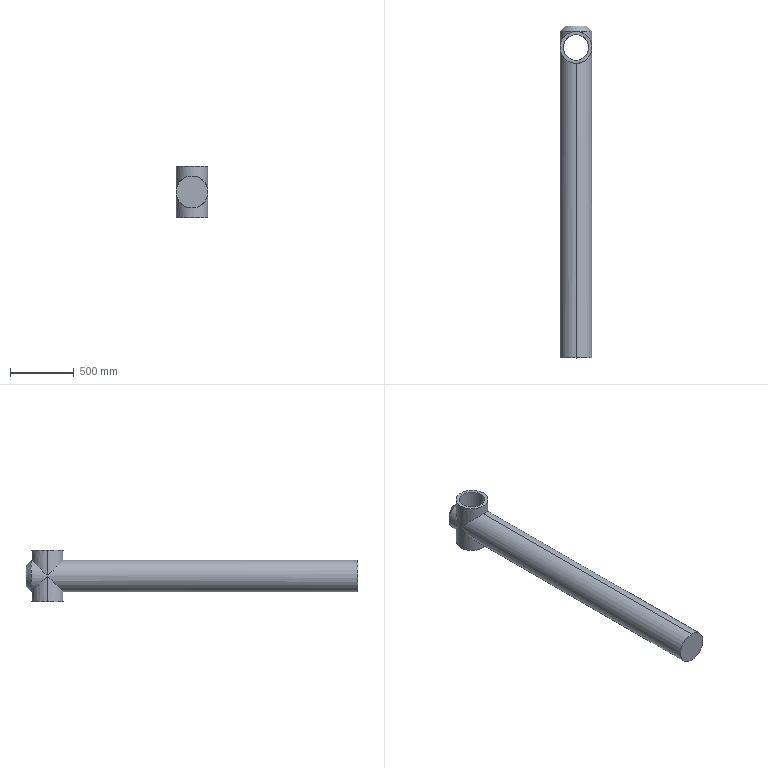Part | SolidWorks | features ICE 3, Chamfer 1, Extrusion 1 | 1 solid | 16 faces | box 250 x 2600 x 400 mm | volume 123717822 mm3 | cylinder 10 | plane 4 | cone 2 | commonest cylinder face diameters 250 x8 200 x2
STEP:
#1=CARTESIAN_POINT('',(0.,4000.,85.));
#2=VERTEX_POINT('',#1);
#3=CARTESIAN_POINT('',(0.,4000.,-85.));
#4=VERTEX_POINT('',#3);
#5=CARTESIAN_POINT('',(0.,4000.,0.));
#6=DIRECTION('',(0.,1.,0.));
#7=DIRECTION('',(0.,0.,1.));
#8=AXIS2_PLACEMENT_3D('',#5,#6,#7);
#9=CIRCLE('',#8,85.);
#10=EDGE_CURVE('',#2,#4,#9,.T.);
#11=ORIENTED_EDGE('',*,*,#10,.F.);
#12=CARTESIAN_POINT('',(0.,3960.,125.));
#13=VERTEX_POINT('',#12);
#14=CARTESIAN_POINT('',(0.,4000.,85.));
#15=DIRECTION('',(0.,-0.7071,0.7071));
#16=VECTOR('',#15,1000.);
#17=LINE('',#14,#16);
#18=EDGE_CURVE('',#2,#13,#17,.T.);
#19=ORIENTED_EDGE('',*,*,#18,.T.);
#20=CARTESIAN_POINT('',(0.,3960.,-125.));
#21=VERTEX_POINT('',#20);
#22=CARTESIAN_POINT('',(0.,3960.,0.));
#23=DIRECTION('',(0.,-1.,0.));
#24=DIRECTION('',(0.,0.,1.));
#25=AXIS2_PLACEMENT_3D('',#22,#23,#24);
#26=CIRCLE('',#25,125.);
#27=EDGE_CURVE('',#21,#13,#26,.T.);
#28=ORIENTED_EDGE('',*,*,#27,.F.);
#29=CARTESIAN_POINT('',(0.,4000.,-85.));
#30=DIRECTION('',(0.,-0.7071,-0.7071));
#31=VECTOR('',#30,1000.);
#32=LINE('',#29,#31);
#33=EDGE_CURVE('',#4,#21,#32,.T.);
#34=ORIENTED_EDGE('',*,*,#33,.F.);
#35=EDGE_LOOP('',(#11,#19,#28,#34));
#36=FACE_OUTER_BOUND('',#35,.T.);
#37=CARTESIAN_POINT('',(0.,4000.,0.));
#38=DIRECTION('',(0.,-1.,0.));
#39=DIRECTION('',(0.,0.,-1.));
#40=AXIS2_PLACEMENT_3D('',#37,#38,#39);
#41=CONICAL_SURFACE('',#40,85.,0.7854);
#42=ADVANCED_FACE('',(#36),#41,.T.);
#43=CARTESIAN_POINT('',(-100.,3832.033,200.));
#44=VERTEX_POINT('',#43);
#45=CARTESIAN_POINT('',(100.,3832.033,200.));
#46=VERTEX_POINT('',#45);
#47=CARTESIAN_POINT('',(0.,3832.033,200.));
#48=DIRECTION('',(0.,0.,1.));
#49=DIRECTION('',(1.,0.,0.));
#50=AXIS2_PLACEMENT_3D('',#47,#48,#49);
#51=CIRCLE('',#50,100.);
#52=EDGE_CURVE('',#44,#46,#51,.T.);
#53=ORIENTED_EDGE('',*,*,#52,.T.);
#54=CARTESIAN_POINT('',(100.,3832.033,-200.));
#55=VERTEX_POINT('',#54);
#56=CARTESIAN_POINT('',(100.,3832.033,4000.));
#57=DIRECTION('',(0.,0.,-1.));
#58=VECTOR('',#57,1000.);
#59=LINE('',#56,#58);
#60=EDGE_CURVE('',#46,#55,#59,.T.);
#61=ORIENTED_EDGE('',*,*,#60,.T.);
#62=CARTESIAN_POINT('',(-100.,3832.033,-200.));
#63=VERTEX_POINT('',#62);
#64=CARTESIAN_POINT('',(0.,3832.033,-200.));
#65=DIRECTION('',(0.,0.,1.));
#66=DIRECTION('',(1.,0.,0.));
#67=AXIS2_PLACEMENT_3D('',#64,#65,#66);
#68=CIRCLE('',#67,100.);
#69=EDGE_CURVE('',#63,#55,#68,.T.);
#70=ORIENTED_EDGE('',*,*,#69,.F.);
#71=CARTESIAN_POINT('',(-100.,3832.033,4000.));
#72=DIRECTION('',(0.,0.,-1.));
#73=VECTOR('',#72,1000.);
#74=LINE('',#71,#73);
#75=EDGE_CURVE('',#44,#63,#74,.T.);
#76=ORIENTED_EDGE('',*,*,#75,.F.);
#77=EDGE_LOOP('',(#53,#61,#70,#76));
#78=FACE_OUTER_BOUND('',#77,.T.);
#79=CARTESIAN_POINT('',(0.,3832.033,4000.));
#80=DIRECTION('',(0.,0.,-1.));
#81=DIRECTION('',(-1.,0.,0.));
#82=AXIS2_PLACEMENT_3D('',#79,#80,#81);
#83=CYLINDRICAL_SURFACE('',#82,100.);
#84=ADVANCED_FACE('',(#78),#83,.F.);
#85=ORIENTED_EDGE('',*,*,#27,.T.);
#86=CARTESIAN_POINT('',(0.,3957.033,125.));
#87=VERTEX_POINT('',#86);
#88=CARTESIAN_POINT('',(0.,4000.,125.));
#89=DIRECTION('',(0.,-1.,0.));
#90=VECTOR('',#89,1000.);
#91=LINE('',#88,#90);
#92=EDGE_CURVE('',#13,#87,#91,.T.);
#93=ORIENTED_EDGE('',*,*,#92,.T.);
#94=CARTESIAN_POINT('',(125.,3832.033,0.));
#95=VERTEX_POINT('',#94);
#96=CARTESIAN_POINT('',(0.,3957.033,125.));
#97=CARTESIAN_POINT('',(73.223,3957.033,125.));
#98=CARTESIAN_POINT('',(125.,3905.257,73.223));
#99=CARTESIAN_POINT('',(125.,3832.033,0.));
#100=(BOUNDED_CURVE()B_SPLINE_CURVE(3,(#96,#97,#98,#99),.UNSPECIFIED.,.F.,.F.)B_SPLINE_CURVE_WITH_KNOTS((4,4),(3.142,4.712),.UNSPECIFIED.)CURVE()GEOMETRIC_REPRESENTATION_ITEM()RATIONAL_B_SPLINE_CURVE((1.,0.8047,0.8047,1.))REPRESENTATION_ITEM(''));
#101=EDGE_CURVE('',#87,#95,#100,.T.);
#102=ORIENTED_EDGE('',*,*,#101,.T.);
#103=CARTESIAN_POINT('',(0.,3957.033,-125.));
#104=VERTEX_POINT('',#103);
#105=CARTESIAN_POINT('',(125.,3832.033,0.));
#106=CARTESIAN_POINT('',(125.,3905.257,-73.223));
#107=CARTESIAN_POINT('',(73.223,3957.033,-125.));
#108=CARTESIAN_POINT('',(0.,3957.033,-125.));
#109=(BOUNDED_CURVE()B_SPLINE_CURVE(3,(#105,#106,#107,#108),.UNSPECIFIED.,.F.,.F.)B_SPLINE_CURVE_WITH_KNOTS((4,4),(1.571,3.142),.UNSPECIFIED.)CURVE()GEOMETRIC_REPRESENTATION_ITEM()RATIONAL_B_SPLINE_CURVE((1.,0.8047,0.8047,1.))REPRESENTATION_ITEM(''));
#110=EDGE_CURVE('',#95,#104,#109,.T.);
#111=ORIENTED_EDGE('',*,*,#110,.T.);
#112=CARTESIAN_POINT('',(0.,4000.,-125.));
#113=DIRECTION('',(0.,-1.,0.));
#114=VECTOR('',#113,1000.);
#115=LINE('',#112,#114);
#116=EDGE_CURVE('',#21,#104,#115,.T.);
#117=ORIENTED_EDGE('',*,*,#116,.F.);
#118=EDGE_LOOP('',(#85,#93,#102,#111,#117));
#119=FACE_OUTER_BOUND('',#118,.T.);
#120=CARTESIAN_POINT('',(0.,4000.,0.));
#121=DIRECTION('',(0.,-1.,0.));
#122=DIRECTION('',(0.,0.,-1.));
#123=AXIS2_PLACEMENT_3D('',#120,#121,#122);
#124=CYLINDRICAL_SURFACE('',#123,125.);
#125=ADVANCED_FACE('',(#119),#124,.T.);
#126=CARTESIAN_POINT('',(125.,3832.033,-200.));
#127=VERTEX_POINT('',#126);
#128=CARTESIAN_POINT('',(-125.,3832.033,-200.));
#129=VERTEX_POINT('',#128);
#130=CARTESIAN_POINT('',(0.,3832.033,-200.));
#131=DIRECTION('',(0.,0.,1.));
#132=DIRECTION('',(1.,0.,0.));
#133=AXIS2_PLACEMENT_3D('',#130,#131,#132);
#134=CIRCLE('',#133,125.);
#135=EDGE_CURVE('',#127,#129,#134,.T.);
#136=ORIENTED_EDGE('',*,*,#135,.T.);
#137=CARTESIAN_POINT('',(-125.,3832.033,0.));
#138=VERTEX_POINT('',#137);
#139=CARTESIAN_POINT('',(-125.,3832.033,-200.));
#140=DIRECTION('',(0.,0.,1.));
#141=VECTOR('',#140,1000.);
#142=LINE('',#139,#141);
#143=EDGE_CURVE('',#129,#138,#142,.T.);
#144=ORIENTED_EDGE('',*,*,#143,.T.);
#145=CARTESIAN_POINT('',(0.,3957.033,-125.));
#146=CARTESIAN_POINT('',(-73.223,3957.033,-125.));
#147=CARTESIAN_POINT('',(-125.,3905.257,-73.223));
#148=CARTESIAN_POINT('',(-125.,3832.033,0.));
#149=(BOUNDED_CURVE()B_SPLINE_CURVE(3,(#145,#146,#147,#148),.UNSPECIFIED.,.F.,.F.)B_SPLINE_CURVE_WITH_KNOTS((4,4),(3.142,4.712),.UNSPECIFIED.)CURVE()GEOMETRIC_REPRESENTATION_ITEM()RATIONAL_B_SPLINE_CURVE((1.,0.8047,0.8047,1.))REPRESENTATION_ITEM(''));
#150=EDGE_CURVE('',#104,#138,#149,.T.);
#151=ORIENTED_EDGE('',*,*,#150,.F.);
#152=ORIENTED_EDGE('',*,*,#110,.F.);
#153=CARTESIAN_POINT('',(125.,3832.033,-200.));
#154=DIRECTION('',(0.,0.,1.));
#155=VECTOR('',#154,1000.);
#156=LINE('',#153,#155);
#157=EDGE_CURVE('',#127,#95,#156,.T.);
#158=ORIENTED_EDGE('',*,*,#157,.F.);
#159=EDGE_LOOP('',(#136,#144,#151,#152,#158));
#160=FACE_OUTER_BOUND('',#159,.T.);
#161=CARTESIAN_POINT('',(0.,3832.033,-200.));
#162=DIRECTION('',(0.,0.,1.));
#163=DIRECTION('',(1.,0.,0.));
#164=AXIS2_PLACEMENT_3D('',#161,#162,#163);
#165=CYLINDRICAL_SURFACE('',#164,125.);
#166=ADVANCED_FACE('',(#160),#165,.T.);
#167=CARTESIAN_POINT('',(-125.,3832.033,0.));
#168=CARTESIAN_POINT('',(-125.,3905.257,73.223));
#169=CARTESIAN_POINT('',(-73.223,3957.033,125.));
#170=CARTESIAN_POINT('',(0.,3957.033,125.));
#171=(BOUNDED_CURVE()B_SPLINE_CURVE(3,(#167,#168,#169,#170),.UNSPECIFIED.,.F.,.F.)B_SPLINE_CURVE_WITH_KNOTS((4,4),(1.571,3.142),.UNSPECIFIED.)CURVE()GEOMETRIC_REPRESENTATION_ITEM()RATIONAL_B_SPLINE_CURVE((1.,0.8047,0.8047,1.))REPRESENTATION_ITEM(''));
#172=EDGE_CURVE('',#138,#87,#171,.T.);
#173=ORIENTED_EDGE('',*,*,#172,.F.);
#174=CARTESIAN_POINT('',(-125.,3832.033,200.));
#175=VERTEX_POINT('',#174);
#176=CARTESIAN_POINT('',(-125.,3832.033,-200.));
#177=DIRECTION('',(0.,0.,1.));
#178=VECTOR('',#177,1000.);
#179=LINE('',#176,#178);
#180=EDGE_CURVE('',#138,#175,#179,.T.);
#181=ORIENTED_EDGE('',*,*,#180,.T.);
#182=CARTESIAN_POINT('',(125.,3832.033,200.));
#183=VERTEX_POINT('',#182);
#184=CARTESIAN_POINT('',(0.,3832.033,200.));
#185=DIRECTION('',(0.,0.,1.));
#186=DIRECTION('',(1.,0.,0.));
#187=AXIS2_PLACEMENT_3D('',#184,#185,#186);
#188=CIRCLE('',#187,125.);
#189=EDGE_CURVE('',#183,#175,#188,.T.);
#190=ORIENTED_EDGE('',*,*,#189,.F.);
#191=CARTESIAN_POINT('',(125.,3832.033,-200.));
#192=DIRECTION('',(0.,0.,1.));
#193=VECTOR('',#192,1000.);
#194=LINE('',#191,#193);
#195=EDGE_CURVE('',#95,#183,#194,.T.);
#196=ORIENTED_EDGE('',*,*,#195,.F.);
#197=ORIENTED_EDGE('',*,*,#101,.F.);
#198=EDGE_LOOP('',(#173,#181,#190,#196,#197));
#199=FACE_OUTER_BOUND('',#198,.T.);
#200=CARTESIAN_POINT('',(0.,3832.033,-200.));
#201=DIRECTION('',(0.,0.,1.));
#202=DIRECTION('',(1.,0.,0.));
#203=AXIS2_PLACEMENT_3D('',#200,#201,#202);
#204=CYLINDRICAL_SURFACE('',#203,125.);
#205=ADVANCED_FACE('',(#199),#204,.T.);
#206=CARTESIAN_POINT('',(0.,3707.033,125.));
#207=VERTEX_POINT('',#206);
#208=CARTESIAN_POINT('',(125.,3832.033,0.));
#209=CARTESIAN_POINT('',(125.,3758.81,73.223));
#210=CARTESIAN_POINT('',(73.223,3707.033,125.));
#211=CARTESIAN_POINT('',(0.,3707.033,125.));
#212=(BOUNDED_CURVE()B_SPLINE_CURVE(3,(#208,#209,#210,#211),.UNSPECIFIED.,.F.,.F.)B_SPLINE_CURVE_WITH_KNOTS((4,4),(4.712,6.283),.UNSPECIFIED.)CURVE()GEOMETRIC_REPRESENTATION_ITEM()RATIONAL_B_SPLINE_CURVE((1.,0.8047,0.8047,1.))REPRESENTATION_ITEM(''));
#213=EDGE_CURVE('',#95,#207,#212,.T.);
#214=ORIENTED_EDGE('',*,*,#213,.T.);
#215=CARTESIAN_POINT('',(0.,1400.,125.));
#216=VERTEX_POINT('',#215);
#217=CARTESIAN_POINT('',(0.,4000.,125.));
#218=DIRECTION('',(0.,-1.,0.));
#219=VECTOR('',#218,1000.);
#220=LINE('',#217,#219);
#221=EDGE_CURVE('',#207,#216,#220,.T.);
#222=ORIENTED_EDGE('',*,*,#221,.T.);
#223=CARTESIAN_POINT('',(0.,1400.,-125.));
#224=VERTEX_POINT('',#223);
#225=CARTESIAN_POINT('',(0.,1400.,0.));
#226=DIRECTION('',(0.,1.,0.));
#227=DIRECTION('',(0.,0.,1.));
#228=AXIS2_PLACEMENT_3D('',#225,#226,#227);
#229=CIRCLE('',#228,125.);
#230=EDGE_CURVE('',#216,#224,#229,.T.);
#231=ORIENTED_EDGE('',*,*,#230,.T.);
#232=CARTESIAN_POINT('',(0.,3707.033,-125.));
#233=VERTEX_POINT('',#232);
#234=CARTESIAN_POINT('',(0.,4000.,-125.));
#235=DIRECTION('',(0.,-1.,0.));
#236=VECTOR('',#235,1000.);
#237=LINE('',#234,#236);
#238=EDGE_CURVE('',#233,#224,#237,.T.);
#239=ORIENTED_EDGE('',*,*,#238,.F.);
#240=CARTESIAN_POINT('',(0.,3707.033,-125.));
#241=CARTESIAN_POINT('',(73.223,3707.033,-125.));
#242=CARTESIAN_POINT('',(125.,3758.81,-73.223));
#243=CARTESIAN_POINT('',(125.,3832.033,0.));
#244=(BOUNDED_CURVE()B_SPLINE_CURVE(3,(#240,#241,#242,#243),.UNSPECIFIED.,.F.,.F.)B_SPLINE_CURVE_WITH_KNOTS((4,4),(0.,1.571),.UNSPECIFIED.)CURVE()GEOMETRIC_REPRESENTATION_ITEM()RATIONAL_B_SPLINE_CURVE((1.,0.8047,0.8047,1.))REPRESENTATION_ITEM(''));
#245=EDGE_CURVE('',#233,#95,#244,.T.);
#246=ORIENTED_EDGE('',*,*,#245,.T.);
#247=EDGE_LOOP('',(#214,#222,#231,#239,#246));
#248=FACE_OUTER_BOUND('',#247,.T.);
#249=CARTESIAN_POINT('',(0.,4000.,0.));
#250=DIRECTION('',(0.,-1.,0.));
#251=DIRECTION('',(0.,0.,-1.));
#252=AXIS2_PLACEMENT_3D('',#249,#250,#251);
#253=CYLINDRICAL_SURFACE('',#252,125.);
#254=ADVANCED_FACE('',(#248),#253,.T.);
#255=ORIENTED_EDGE('',*,*,#221,.F.);
#256=CARTESIAN_POINT('',(0.,3707.033,125.));
#257=CARTESIAN_POINT('',(-73.223,3707.033,125.));
#258=CARTESIAN_POINT('',(-125.,3758.81,73.223));
#259=CARTESIAN_POINT('',(-125.,3832.033,0.));
#260=(BOUNDED_CURVE()B_SPLINE_CURVE(3,(#256,#257,#258,#259),.UNSPECIFIED.,.F.,.F.)B_SPLINE_CURVE_WITH_KNOTS((4,4),(0.,1.571),.UNSPECIFIED.)CURVE()GEOMETRIC_REPRESENTATION_ITEM()RATIONAL_B_SPLINE_CURVE((1.,0.8047,0.8047,1.))REPRESENTATION_ITEM(''));
#261=EDGE_CURVE('',#207,#138,#260,.T.);
#262=ORIENTED_EDGE('',*,*,#261,.T.);
#263=CARTESIAN_POINT('',(-125.,3832.033,0.));
#264=CARTESIAN_POINT('',(-125.,3758.81,-73.223));
#265=CARTESIAN_POINT('',(-73.223,3707.033,-125.));
#266=CARTESIAN_POINT('',(0.,3707.033,-125.));
#267=(BOUNDED_CURVE()B_SPLINE_CURVE(3,(#263,#264,#265,#266),.UNSPECIFIED.,.F.,.F.)B_SPLINE_CURVE_WITH_KNOTS((4,4),(4.712,6.283),.UNSPECIFIED.)CURVE()GEOMETRIC_REPRESENTATION_ITEM()RATIONAL_B_SPLINE_CURVE((1.,0.8047,0.8047,1.))REPRESENTATION_ITEM(''));
#268=EDGE_CURVE('',#138,#233,#267,.T.);
#269=ORIENTED_EDGE('',*,*,#268,.T.);
#270=ORIENTED_EDGE('',*,*,#238,.T.);
#271=CARTESIAN_POINT('',(0.,1400.,0.));
#272=DIRECTION('',(0.,1.,0.));
#273=DIRECTION('',(0.,0.,1.));
#274=AXIS2_PLACEMENT_3D('',#271,#272,#273);
#275=CIRCLE('',#274,125.);
#276=EDGE_CURVE('',#224,#216,#275,.T.);
#277=ORIENTED_EDGE('',*,*,#276,.T.);
#278=EDGE_LOOP('',(#255,#262,#269,#270,#277));
#279=FACE_OUTER_BOUND('',#278,.T.);
#280=CARTESIAN_POINT('',(0.,4000.,0.));
#281=DIRECTION('',(0.,-1.,0.));
#282=DIRECTION('',(0.,0.,-1.));
#283=AXIS2_PLACEMENT_3D('',#280,#281,#282);
#284=CYLINDRICAL_SURFACE('',#283,125.);
#285=ADVANCED_FACE('',(#279),#284,.T.);
#286=ORIENTED_EDGE('',*,*,#276,.F.);
#287=ORIENTED_EDGE('',*,*,#230,.F.);
#288=EDGE_LOOP('',(#286,#287));
#289=FACE_OUTER_BOUND('',#288,.T.);
#290=CARTESIAN_POINT('',(0.,1400.,0.));
#291=DIRECTION('',(0.,1.,0.));
#292=DIRECTION('',(0.,0.,1.));
#293=AXIS2_PLACEMENT_3D('',#290,#291,#292);
#294=PLANE('',#293);
#295=ADVANCED_FACE('',(#289),#294,.F.);
#296=ORIENTED_EDGE('',*,*,#180,.F.);
#297=ORIENTED_EDGE('',*,*,#261,.F.);
#298=ORIENTED_EDGE('',*,*,#213,.F.);
#299=ORIENTED_EDGE('',*,*,#195,.T.);
#300=CARTESIAN_POINT('',(0.,3832.033,200.));
#301=DIRECTION('',(0.,0.,1.));
#302=DIRECTION('',(1.,0.,0.));
#303=AXIS2_PLACEMENT_3D('',#300,#301,#302);
#304=CIRCLE('',#303,125.);
#305=EDGE_CURVE('',#175,#183,#304,.T.);
#306=ORIENTED_EDGE('',*,*,#305,.F.);
#307=EDGE_LOOP('',(#296,#297,#298,#299,#306));
#308=FACE_OUTER_BOUND('',#307,.T.);
#309=CARTESIAN_POINT('',(0.,3832.033,-200.));
#310=DIRECTION('',(0.,0.,1.));
#311=DIRECTION('',(1.,0.,0.));
#312=AXIS2_PLACEMENT_3D('',#309,#310,#311);
#313=CYLINDRICAL_SURFACE('',#312,125.);
#314=ADVANCED_FACE('',(#308),#313,.T.);
#315=ORIENTED_EDGE('',*,*,#189,.T.);
#316=ORIENTED_EDGE('',*,*,#305,.T.);
#317=EDGE_LOOP('',(#315,#316));
#318=FACE_OUTER_BOUND('',#317,.T.);
#319=ORIENTED_EDGE('',*,*,#52,.F.);
#320=CARTESIAN_POINT('',(0.,3832.033,200.));
#321=DIRECTION('',(0.,0.,1.));
#322=DIRECTION('',(1.,0.,0.));
#323=AXIS2_PLACEMENT_3D('',#320,#321,#322);
#324=CIRCLE('',#323,100.);
#325=EDGE_CURVE('',#46,#44,#324,.T.);
#326=ORIENTED_EDGE('',*,*,#325,.F.);
#327=EDGE_LOOP('',(#319,#326));
#328=FACE_BOUND('',#327,.T.);
#329=CARTESIAN_POINT('',(0.,3832.033,200.));
#330=DIRECTION('',(0.,0.,1.));
#331=DIRECTION('',(1.,0.,0.));
#332=AXIS2_PLACEMENT_3D('',#329,#330,#331);
#333=PLANE('',#332);
#334=ADVANCED_FACE('',(#318,#328),#333,.T.);
#335=ORIENTED_EDGE('',*,*,#143,.F.);
#336=CARTESIAN_POINT('',(0.,3832.033,-200.));
#337=DIRECTION('',(0.,0.,1.));
#338=DIRECTION('',(1.,0.,0.));
#339=AXIS2_PLACEMENT_3D('',#336,#337,#338);
#340=CIRCLE('',#339,125.);
#341=EDGE_CURVE('',#129,#127,#340,.T.);
#342=ORIENTED_EDGE('',*,*,#341,.T.);
#343=ORIENTED_EDGE('',*,*,#157,.T.);
#344=ORIENTED_EDGE('',*,*,#245,.F.);
#345=ORIENTED_EDGE('',*,*,#268,.F.);
#346=EDGE_LOOP('',(#335,#342,#343,#344,#345));
#347=FACE_OUTER_BOUND('',#346,.T.);
#348=CARTESIAN_POINT('',(0.,3832.033,-200.));
#349=DIRECTION('',(0.,0.,1.));
#350=DIRECTION('',(1.,0.,0.));
#351=AXIS2_PLACEMENT_3D('',#348,#349,#350);
#352=CYLINDRICAL_SURFACE('',#351,125.);
#353=ADVANCED_FACE('',(#347),#352,.T.);
#354=ORIENTED_EDGE('',*,*,#69,.T.);
#355=CARTESIAN_POINT('',(0.,3832.033,-200.));
#356=DIRECTION('',(0.,0.,1.));
#357=DIRECTION('',(1.,0.,0.));
#358=AXIS2_PLACEMENT_3D('',#355,#356,#357);
#359=CIRCLE('',#358,100.);
#360=EDGE_CURVE('',#55,#63,#359,.T.);
#361=ORIENTED_EDGE('',*,*,#360,.T.);
#362=EDGE_LOOP('',(#354,#361));
#363=FACE_BOUND('',#362,.T.);
#364=ORIENTED_EDGE('',*,*,#135,.F.);
#365=ORIENTED_EDGE('',*,*,#341,.F.);
#366=EDGE_LOOP('',(#364,#365));
#367=FACE_OUTER_BOUND('',#366,.T.);
#368=CARTESIAN_POINT('',(0.,3832.033,-200.));
#369=DIRECTION('',(0.,0.,1.));
#370=DIRECTION('',(1.,0.,0.));
#371=AXIS2_PLACEMENT_3D('',#368,#369,#370);
#372=PLANE('',#371);
#373=ADVANCED_FACE('',(#363,#367),#372,.F.);
#374=CARTESIAN_POINT('',(0.,4000.,0.));
#375=DIRECTION('',(0.,1.,0.));
#376=DIRECTION('',(0.,0.,1.));
#377=AXIS2_PLACEMENT_3D('',#374,#375,#376);
#378=CIRCLE('',#377,85.);
#379=EDGE_CURVE('',#4,#2,#378,.T.);
#380=ORIENTED_EDGE('',*,*,#379,.T.);
#381=ORIENTED_EDGE('',*,*,#10,.T.);
#382=EDGE_LOOP('',(#380,#381));
#383=FACE_OUTER_BOUND('',#382,.T.);
#384=CARTESIAN_POINT('',(0.,4000.,0.));
#385=DIRECTION('',(0.,1.,0.));
#386=DIRECTION('',(0.,0.,1.));
#387=AXIS2_PLACEMENT_3D('',#384,#385,#386);
#388=PLANE('',#387);
#389=ADVANCED_FACE('',(#383),#388,.T.);
#390=ORIENTED_EDGE('',*,*,#92,.F.);
#391=CARTESIAN_POINT('',(0.,3960.,0.));
#392=DIRECTION('',(0.,-1.,0.));
#393=DIRECTION('',(0.,0.,1.));
#394=AXIS2_PLACEMENT_3D('',#391,#392,#393);
#395=CIRCLE('',#394,125.);
#396=EDGE_CURVE('',#13,#21,#395,.T.);
#397=ORIENTED_EDGE('',*,*,#396,.T.);
#398=ORIENTED_EDGE('',*,*,#116,.T.);
#399=ORIENTED_EDGE('',*,*,#150,.T.);
#400=ORIENTED_EDGE('',*,*,#172,.T.);
#401=EDGE_LOOP('',(#390,#397,#398,#399,#400));
#402=FACE_OUTER_BOUND('',#401,.T.);
#403=CARTESIAN_POINT('',(0.,4000.,0.));
#404=DIRECTION('',(0.,-1.,0.));
#405=DIRECTION('',(0.,0.,-1.));
#406=AXIS2_PLACEMENT_3D('',#403,#404,#405);
#407=CYLINDRICAL_SURFACE('',#406,125.);
#408=ADVANCED_FACE('',(#402),#407,.T.);
#409=ORIENTED_EDGE('',*,*,#60,.F.);
#410=ORIENTED_EDGE('',*,*,#325,.T.);
#411=ORIENTED_EDGE('',*,*,#75,.T.);
#412=ORIENTED_EDGE('',*,*,#360,.F.);
#413=EDGE_LOOP('',(#409,#410,#411,#412));
#414=FACE_OUTER_BOUND('',#413,.T.);
#415=CARTESIAN_POINT('',(0.,3832.033,4000.));
#416=DIRECTION('',(0.,0.,-1.));
#417=DIRECTION('',(-1.,0.,0.));
#418=AXIS2_PLACEMENT_3D('',#415,#416,#417);
#419=CYLINDRICAL_SURFACE('',#418,100.);
#420=ADVANCED_FACE('',(#414),#419,.F.);
#421=ORIENTED_EDGE('',*,*,#18,.F.);
#422=ORIENTED_EDGE('',*,*,#379,.F.);
#423=ORIENTED_EDGE('',*,*,#33,.T.);
#424=ORIENTED_EDGE('',*,*,#396,.F.);
#425=EDGE_LOOP('',(#421,#422,#423,#424));
#426=FACE_OUTER_BOUND('',#425,.T.);
#427=CARTESIAN_POINT('',(0.,4000.,0.));
#428=DIRECTION('',(0.,-1.,0.));
#429=DIRECTION('',(0.,0.,-1.));
#430=AXIS2_PLACEMENT_3D('',#427,#428,#429);
#431=CONICAL_SURFACE('',#430,85.,0.7854);
#432=ADVANCED_FACE('',(#426),#431,.T.);
#433=CLOSED_SHELL('',(#42,#84,#125,#166,#205,#254,#285,#295,#314,#334,#353,#373,#389,#408,#420,#432));
#434=MANIFOLD_SOLID_BREP('',#433);
#435=CARTESIAN_POINT('',(0.,0.,0.));
#436=DIRECTION('',(0.,0.,1.));
#437=DIRECTION('',(1.,0.,0.));
#438=AXIS2_PLACEMENT_3D('',#435,#436,#437);
#439=(LENGTH_UNIT()NAMED_UNIT(*)SI_UNIT(.MILLI.,.METRE.));
#440=UNCERTAINTY_MEASURE_WITH_UNIT(LENGTH_MEASURE(0.00001),#439,'','');
#441=(NAMED_UNIT(*)PLANE_ANGLE_UNIT()SI_UNIT($,.RADIAN.));
#442=(NAMED_UNIT(*)SI_UNIT($,.STERADIAN.)SOLID_ANGLE_UNIT());
#443=(GEOMETRIC_REPRESENTATION_CONTEXT(3)GLOBAL_UNCERTAINTY_ASSIGNED_CONTEXT((#440))GLOBAL_UNIT_ASSIGNED_CONTEXT((#439,#441,#442))REPRESENTATION_CONTEXT('',''));
#444=ADVANCED_BREP_SHAPE_REPRESENTATION('',(#434,#438),#443);